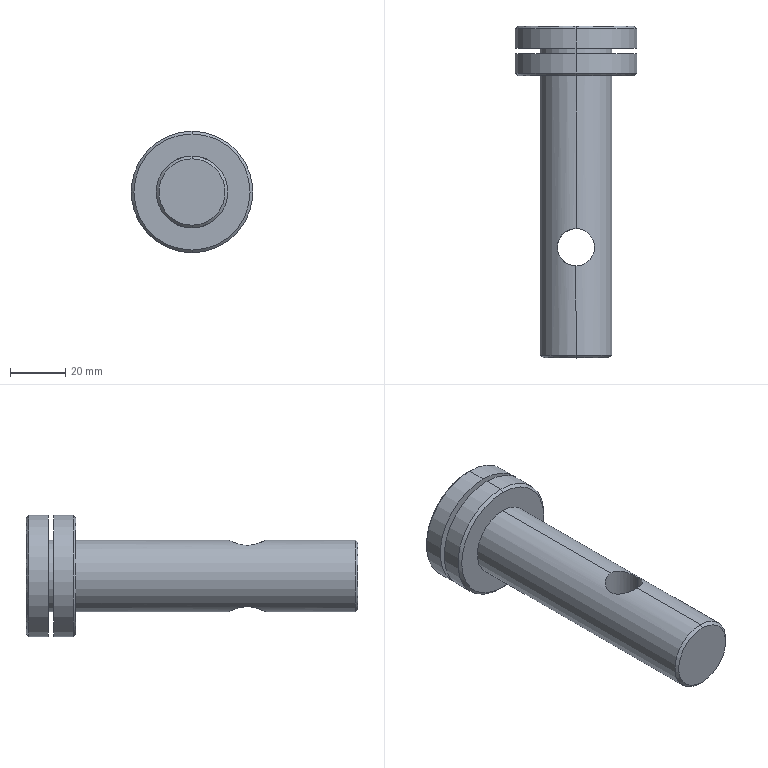Part | SolidWorks | features 3DProfileFeature 1, Chamfer 1, CirPattern 1, HoleWzd 1, ICE 1, Revolution 1 | 1 solid | 37 faces | box 44 x 120 x 44 mm | volume 75501 mm3 | cylinder 18 | cone 14 | plane 5 | commonest cylinder face diameters 3.3 x8 26 x4 44 x4 13.5 x2
STEP:
#1=CARTESIAN_POINT('',(-6.75,40.,-11.11));
#2=VERTEX_POINT('',#1);
#3=CARTESIAN_POINT('',(0.,33.25,-13.));
#4=VERTEX_POINT('',#3);
#5=CARTESIAN_POINT('',(-6.75,40.,-11.11));
#6=CARTESIAN_POINT('',(-6.75,39.775,-11.11));
#7=CARTESIAN_POINT('',(-6.739,39.547,-11.117));
#8=CARTESIAN_POINT('',(-6.693,39.098,-11.145));
#9=CARTESIAN_POINT('',(-6.66,38.877,-11.165));
#10=CARTESIAN_POINT('',(-6.571,38.44,-11.217));
#11=CARTESIAN_POINT('',(-6.516,38.224,-11.249));
#12=CARTESIAN_POINT('',(-6.385,37.799,-11.324));
#13=CARTESIAN_POINT('',(-6.308,37.589,-11.367));
#14=CARTESIAN_POINT('',(-6.051,36.977,-11.507));
#15=CARTESIAN_POINT('',(-5.844,36.593,-11.616));
#16=CARTESIAN_POINT('',(-5.478,36.051,-11.79));
#17=CARTESIAN_POINT('',(-5.347,35.874,-11.85));
#18=CARTESIAN_POINT('',(-5.07,35.539,-11.971));
#19=CARTESIAN_POINT('',(-4.925,35.379,-12.032));
#20=CARTESIAN_POINT('',(-4.466,34.92,-12.213));
#21=CARTESIAN_POINT('',(-4.132,34.644,-12.332));
#22=CARTESIAN_POINT('',(-3.4,34.152,-12.553));
#23=CARTESIAN_POINT('',(-3.015,33.945,-12.652));
#24=CARTESIAN_POINT('',(-2.408,33.69,-12.777));
#25=CARTESIAN_POINT('',(-2.2,33.615,-12.814));
#26=CARTESIAN_POINT('',(-1.775,33.484,-12.88));
#27=CARTESIAN_POINT('',(-1.555,33.428,-12.909));
#28=CARTESIAN_POINT('',(-0.8938,33.294,-12.977));
#29=CARTESIAN_POINT('',(-0.4489,33.25,-13.));
#30=CARTESIAN_POINT('',(0.,33.25,-13.));
#31=B_SPLINE_CURVE_WITH_KNOTS('',3,(#5,#6,#7,#8,#9,#10,#11,#12,#13,#14,#15,#16,#17,#18,#19,#20,#21,#22,#23,#24,#25,#26,#27,#28,#29,#30),.UNSPECIFIED.,.F.,.F.,(4,2,2,2,2,2,2,2,2,2,2,2,4),(0.01076,0.01143,0.0121,0.01277,0.01345,0.01479,0.01546,0.01613,0.01747,0.01882,0.01949,0.02016,0.0215),.UNSPECIFIED.);
#32=EDGE_CURVE('',#2,#4,#31,.T.);
#33=ORIENTED_EDGE('',*,*,#32,.F.);
#34=CARTESIAN_POINT('',(-6.75,40.,11.11));
#35=VERTEX_POINT('',#34);
#36=CARTESIAN_POINT('',(-6.75,40.,-22.));
#37=DIRECTION('',(0.,0.,1.));
#38=VECTOR('',#37,1000.);
#39=LINE('',#36,#38);
#40=EDGE_CURVE('',#2,#35,#39,.T.);
#41=ORIENTED_EDGE('',*,*,#40,.T.);
#42=CARTESIAN_POINT('',(0.,33.25,13.));
#43=VERTEX_POINT('',#42);
#44=CARTESIAN_POINT('',(0.,33.25,13.));
#45=CARTESIAN_POINT('',(-0.2253,33.25,13.));
#46=CARTESIAN_POINT('',(-0.4536,33.261,12.994));
#47=CARTESIAN_POINT('',(-0.9024,33.307,12.971));
#48=CARTESIAN_POINT('',(-1.124,33.34,12.953));
#49=CARTESIAN_POINT('',(-1.561,33.429,12.908));
#50=CARTESIAN_POINT('',(-1.777,33.484,12.88));
#51=CARTESIAN_POINT('',(-2.204,33.616,12.814));
#52=CARTESIAN_POINT('',(-2.415,33.693,12.775));
#53=CARTESIAN_POINT('',(-3.029,33.951,12.649));
#54=CARTESIAN_POINT('',(-3.414,34.161,12.549));
#55=CARTESIAN_POINT('',(-3.958,34.528,12.384));
#56=CARTESIAN_POINT('',(-4.134,34.66,12.326));
#57=CARTESIAN_POINT('',(-4.471,34.938,12.208));
#58=CARTESIAN_POINT('',(-4.631,35.084,12.148));
#59=CARTESIAN_POINT('',(-5.088,35.544,11.967));
#60=CARTESIAN_POINT('',(-5.363,35.878,11.845));
#61=CARTESIAN_POINT('',(-5.852,36.607,11.612));
#62=CARTESIAN_POINT('',(-6.058,36.991,11.504));
#63=CARTESIAN_POINT('',(-6.311,37.597,11.366));
#64=CARTESIAN_POINT('',(-6.386,37.803,11.323));
#65=CARTESIAN_POINT('',(-6.517,38.228,11.249));
#66=CARTESIAN_POINT('',(-6.573,38.447,11.216));
#67=CARTESIAN_POINT('',(-6.706,39.107,11.137));
#68=CARTESIAN_POINT('',(-6.75,39.552,11.11));
#69=CARTESIAN_POINT('',(-6.75,40.,11.11));
#70=B_SPLINE_CURVE_WITH_KNOTS('',3,(#44,#45,#46,#47,#48,#49,#50,#51,#52,#53,#54,#55,#56,#57,#58,#59,#60,#61,#62,#63,#64,#65,#66,#67,#68,#69),.UNSPECIFIED.,.F.,.F.,(4,2,2,2,2,2,2,2,2,2,2,2,4),(0.01076,0.01143,0.0121,0.01277,0.01344,0.01479,0.01546,0.01613,0.01747,0.01881,0.01949,0.02016,0.0215),.UNSPECIFIED.);
#71=EDGE_CURVE('',#43,#35,#70,.T.);
#72=ORIENTED_EDGE('',*,*,#71,.F.);
#73=CARTESIAN_POINT('',(6.75,40.,11.11));
#74=VERTEX_POINT('',#73);
#75=CARTESIAN_POINT('',(6.75,40.,11.11));
#76=CARTESIAN_POINT('',(6.75,39.545,11.11));
#77=CARTESIAN_POINT('',(6.704,39.099,11.138));
#78=CARTESIAN_POINT('',(6.528,38.225,11.243));
#79=CARTESIAN_POINT('',(6.394,37.793,11.32));
#80=CARTESIAN_POINT('',(6.053,36.981,11.506));
#81=CARTESIAN_POINT('',(5.846,36.597,11.615));
#82=CARTESIAN_POINT('',(5.357,35.87,11.848));
#83=CARTESIAN_POINT('',(5.08,35.534,11.971));
#84=CARTESIAN_POINT('',(4.621,35.075,12.152));
#85=CARTESIAN_POINT('',(4.461,34.929,12.212));
#86=CARTESIAN_POINT('',(4.125,34.652,12.33));
#87=CARTESIAN_POINT('',(3.948,34.52,12.388));
#88=CARTESIAN_POINT('',(3.402,34.154,12.553));
#89=CARTESIAN_POINT('',(3.018,33.946,12.652));
#90=CARTESIAN_POINT('',(2.409,33.691,12.776));
#91=CARTESIAN_POINT('',(2.201,33.615,12.814));
#92=CARTESIAN_POINT('',(1.772,33.483,12.88));
#93=CARTESIAN_POINT('',(1.553,33.427,12.909));
#94=CARTESIAN_POINT('',(0.8956,33.295,12.977));
#95=CARTESIAN_POINT('',(0.451,33.25,13.));
#96=CARTESIAN_POINT('',(0.,33.25,13.));
#97=B_SPLINE_CURVE_WITH_KNOTS('',3,(#75,#76,#77,#78,#79,#80,#81,#82,#83,#84,#85,#86,#87,#88,#89,#90,#91,#92,#93,#94,#95,#96),.UNSPECIFIED.,.F.,.F.,(4,2,2,2,2,2,2,2,2,2,4),(0.,0.001344,0.002689,0.004033,0.005378,0.00605,0.006722,0.008066,0.008739,0.009411,0.01076),.UNSPECIFIED.);
#98=EDGE_CURVE('',#74,#43,#97,.T.);
#99=ORIENTED_EDGE('',*,*,#98,.F.);
#100=CARTESIAN_POINT('',(6.75,40.,-11.11));
#101=VERTEX_POINT('',#100);
#102=CARTESIAN_POINT('',(6.75,40.,-22.));
#103=DIRECTION('',(0.,0.,1.));
#104=VECTOR('',#103,1000.);
#105=LINE('',#102,#104);
#106=EDGE_CURVE('',#101,#74,#105,.T.);
#107=ORIENTED_EDGE('',*,*,#106,.F.);
#108=CARTESIAN_POINT('',(0.,33.25,-13.));
#109=CARTESIAN_POINT('',(0.4487,33.25,-13.));
#110=CARTESIAN_POINT('',(0.9051,33.296,-12.976));
#111=CARTESIAN_POINT('',(1.781,33.474,-12.885));
#112=CARTESIAN_POINT('',(2.207,33.605,-12.818));
#113=CARTESIAN_POINT('',(3.029,33.951,-12.649));
#114=CARTESIAN_POINT('',(3.414,34.161,-12.549));
#115=CARTESIAN_POINT('',(4.138,34.649,-12.33));
#116=CARTESIAN_POINT('',(4.478,34.93,-12.209));
#117=CARTESIAN_POINT('',(5.089,35.544,-11.967));
#118=CARTESIAN_POINT('',(5.363,35.878,-11.845));
#119=CARTESIAN_POINT('',(5.728,36.422,-11.671));
#120=CARTESIAN_POINT('',(5.842,36.611,-11.614));
#121=CARTESIAN_POINT('',(6.049,36.996,-11.508));
#122=CARTESIAN_POINT('',(6.143,37.194,-11.458));
#123=CARTESIAN_POINT('',(6.396,37.799,-11.319));
#124=CARTESIAN_POINT('',(6.527,38.22,-11.243));
#125=CARTESIAN_POINT('',(6.706,39.105,-11.138));
#126=CARTESIAN_POINT('',(6.75,39.553,-11.11));
#127=CARTESIAN_POINT('',(6.75,40.,-11.11));
#128=B_SPLINE_CURVE_WITH_KNOTS('',3,(#108,#109,#110,#111,#112,#113,#114,#115,#116,#117,#118,#119,#120,#121,#122,#123,#124,#125,#126,#127),.UNSPECIFIED.,.F.,.F.,(4,2,2,2,2,2,2,2,2,4),(0.0215,0.02285,0.02419,0.02553,0.02687,0.02822,0.02889,0.02956,0.0309,0.03224),.UNSPECIFIED.);
#129=EDGE_CURVE('',#4,#101,#128,.T.);
#130=ORIENTED_EDGE('',*,*,#129,.F.);
#131=EDGE_LOOP('',(#33,#41,#72,#99,#107,#130));
#132=FACE_OUTER_BOUND('',#131,.T.);
#133=CARTESIAN_POINT('',(0.,40.,-22.));
#134=DIRECTION('',(0.,0.,1.));
#135=DIRECTION('',(1.,0.,0.));
#136=AXIS2_PLACEMENT_3D('',#133,#134,#135);
#137=CYLINDRICAL_SURFACE('',#136,6.75);
#138=ADVANCED_FACE('',(#132),#137,.F.);
#139=CARTESIAN_POINT('',(15.,119.625,-1.65));
#140=VERTEX_POINT('',#139);
#141=CARTESIAN_POINT('',(15.,119.625,1.65));
#142=VERTEX_POINT('',#141);
#143=CARTESIAN_POINT('',(15.,119.625,0.));
#144=DIRECTION('',(0.,1.,0.));
#145=DIRECTION('',(0.,0.,1.));
#146=AXIS2_PLACEMENT_3D('',#143,#144,#145);
#147=CIRCLE('',#146,1.65);
#148=EDGE_CURVE('',#140,#142,#147,.T.);
#149=ORIENTED_EDGE('',*,*,#148,.F.);
#150=CARTESIAN_POINT('',(15.,120.,-2.025));
#151=VERTEX_POINT('',#150);
#152=CARTESIAN_POINT('',(15.,120.,-2.025));
#153=DIRECTION('',(0.,0.7071,-0.7071));
#154=VECTOR('',#153,1000.);
#155=LINE('',#152,#154);
#156=EDGE_CURVE('',#140,#151,#155,.T.);
#157=ORIENTED_EDGE('',*,*,#156,.T.);
#158=CARTESIAN_POINT('',(15.,120.,2.025));
#159=VERTEX_POINT('',#158);
#160=CARTESIAN_POINT('',(15.,120.,0.));
#161=DIRECTION('',(0.,1.,0.));
#162=DIRECTION('',(0.,0.,1.));
#163=AXIS2_PLACEMENT_3D('',#160,#161,#162);
#164=CIRCLE('',#163,2.025);
#165=EDGE_CURVE('',#151,#159,#164,.T.);
#166=ORIENTED_EDGE('',*,*,#165,.T.);
#167=CARTESIAN_POINT('',(15.,120.,2.025));
#168=DIRECTION('',(0.,0.7071,0.7071));
#169=VECTOR('',#168,1000.);
#170=LINE('',#167,#169);
#171=EDGE_CURVE('',#142,#159,#170,.T.);
#172=ORIENTED_EDGE('',*,*,#171,.F.);
#173=EDGE_LOOP('',(#149,#157,#166,#172));
#174=FACE_OUTER_BOUND('',#173,.T.);
#175=CARTESIAN_POINT('',(15.,120.,0.));
#176=DIRECTION('',(0.,1.,0.));
#177=DIRECTION('',(0.,0.,1.));
#178=AXIS2_PLACEMENT_3D('',#175,#176,#177);
#179=CONICAL_SURFACE('',#178,2.025,0.7854);
#180=ADVANCED_FACE('',(#174),#179,.F.);
#181=CARTESIAN_POINT('',(15.,112.,-1.65));
#182=VERTEX_POINT('',#181);
#183=CARTESIAN_POINT('',(15.,112.,1.65));
#184=VERTEX_POINT('',#183);
#185=CARTESIAN_POINT('',(15.,112.,0.));
#186=DIRECTION('',(0.,1.,0.));
#187=DIRECTION('',(0.,0.,1.));
#188=AXIS2_PLACEMENT_3D('',#185,#186,#187);
#189=CIRCLE('',#188,1.65);
#190=EDGE_CURVE('',#182,#184,#189,.T.);
#191=ORIENTED_EDGE('',*,*,#190,.F.);
#192=CARTESIAN_POINT('',(15.,120.,-1.65));
#193=DIRECTION('',(0.,1.,0.));
#194=VECTOR('',#193,1000.);
#195=LINE('',#192,#194);
#196=EDGE_CURVE('',#182,#140,#195,.T.);
#197=ORIENTED_EDGE('',*,*,#196,.T.);
#198=ORIENTED_EDGE('',*,*,#148,.T.);
#199=CARTESIAN_POINT('',(15.,120.,1.65));
#200=DIRECTION('',(0.,1.,0.));
#201=VECTOR('',#200,1000.);
#202=LINE('',#199,#201);
#203=EDGE_CURVE('',#184,#142,#202,.T.);
#204=ORIENTED_EDGE('',*,*,#203,.F.);
#205=EDGE_LOOP('',(#191,#197,#198,#204));
#206=FACE_OUTER_BOUND('',#205,.T.);
#207=CARTESIAN_POINT('',(15.,120.,0.));
#208=DIRECTION('',(0.,1.,0.));
#209=DIRECTION('',(0.,0.,1.));
#210=AXIS2_PLACEMENT_3D('',#207,#208,#209);
#211=CYLINDRICAL_SURFACE('',#210,1.65);
#212=ADVANCED_FACE('',(#206),#211,.F.);
#213=CARTESIAN_POINT('',(0.,119.625,13.35));
#214=VERTEX_POINT('',#213);
#215=CARTESIAN_POINT('',(0.,119.625,16.65));
#216=VERTEX_POINT('',#215);
#217=CARTESIAN_POINT('',(0.,119.625,15.));
#218=DIRECTION('',(0.,1.,0.));
#219=DIRECTION('',(0.,0.,1.));
#220=AXIS2_PLACEMENT_3D('',#217,#218,#219);
#221=CIRCLE('',#220,1.65);
#222=EDGE_CURVE('',#214,#216,#221,.T.);
#223=ORIENTED_EDGE('',*,*,#222,.F.);
#224=CARTESIAN_POINT('',(0.,120.,12.975));
#225=VERTEX_POINT('',#224);
#226=CARTESIAN_POINT('',(0.,120.,12.975));
#227=DIRECTION('',(0.,0.7071,-0.7071));
#228=VECTOR('',#227,1000.);
#229=LINE('',#226,#228);
#230=EDGE_CURVE('',#214,#225,#229,.T.);
#231=ORIENTED_EDGE('',*,*,#230,.T.);
#232=CARTESIAN_POINT('',(0.,120.,17.025));
#233=VERTEX_POINT('',#232);
#234=CARTESIAN_POINT('',(0.,120.,15.));
#235=DIRECTION('',(0.,1.,0.));
#236=DIRECTION('',(0.,0.,1.));
#237=AXIS2_PLACEMENT_3D('',#234,#235,#236);
#238=CIRCLE('',#237,2.025);
#239=EDGE_CURVE('',#225,#233,#238,.T.);
#240=ORIENTED_EDGE('',*,*,#239,.T.);
#241=CARTESIAN_POINT('',(0.,120.,17.025));
#242=DIRECTION('',(0.,0.7071,0.7071));
#243=VECTOR('',#242,1000.);
#244=LINE('',#241,#243);
#245=EDGE_CURVE('',#216,#233,#244,.T.);
#246=ORIENTED_EDGE('',*,*,#245,.F.);
#247=EDGE_LOOP('',(#223,#231,#240,#246));
#248=FACE_OUTER_BOUND('',#247,.T.);
#249=CARTESIAN_POINT('',(0.,120.,15.));
#250=DIRECTION('',(0.,1.,0.));
#251=DIRECTION('',(0.,0.,1.));
#252=AXIS2_PLACEMENT_3D('',#249,#250,#251);
#253=CONICAL_SURFACE('',#252,2.025,0.7854);
#254=ADVANCED_FACE('',(#248),#253,.F.);
#255=CARTESIAN_POINT('',(0.,112.,13.35));
#256=VERTEX_POINT('',#255);
#257=CARTESIAN_POINT('',(0.,112.,16.65));
#258=VERTEX_POINT('',#257);
#259=CARTESIAN_POINT('',(0.,112.,15.));
#260=DIRECTION('',(0.,1.,0.));
#261=DIRECTION('',(0.,0.,1.));
#262=AXIS2_PLACEMENT_3D('',#259,#260,#261);
#263=CIRCLE('',#262,1.65);
#264=EDGE_CURVE('',#256,#258,#263,.T.);
#265=ORIENTED_EDGE('',*,*,#264,.F.);
#266=CARTESIAN_POINT('',(0.,120.,13.35));
#267=DIRECTION('',(0.,1.,0.));
#268=VECTOR('',#267,1000.);
#269=LINE('',#266,#268);
#270=EDGE_CURVE('',#256,#214,#269,.T.);
#271=ORIENTED_EDGE('',*,*,#270,.T.);
#272=ORIENTED_EDGE('',*,*,#222,.T.);
#273=CARTESIAN_POINT('',(0.,120.,16.65));
#274=DIRECTION('',(0.,1.,0.));
#275=VECTOR('',#274,1000.);
#276=LINE('',#273,#275);
#277=EDGE_CURVE('',#258,#216,#276,.T.);
#278=ORIENTED_EDGE('',*,*,#277,.F.);
#279=EDGE_LOOP('',(#265,#271,#272,#278));
#280=FACE_OUTER_BOUND('',#279,.T.);
#281=CARTESIAN_POINT('',(0.,120.,15.));
#282=DIRECTION('',(0.,1.,0.));
#283=DIRECTION('',(0.,0.,1.));
#284=AXIS2_PLACEMENT_3D('',#281,#282,#283);
#285=CYLINDRICAL_SURFACE('',#284,1.65);
#286=ADVANCED_FACE('',(#280),#285,.F.);
#287=CARTESIAN_POINT('',(-15.,119.625,-1.65));
#288=VERTEX_POINT('',#287);
#289=CARTESIAN_POINT('',(-15.,119.625,1.65));
#290=VERTEX_POINT('',#289);
#291=CARTESIAN_POINT('',(-15.,119.625,0.));
#292=DIRECTION('',(0.,1.,0.));
#293=DIRECTION('',(0.,0.,1.));
#294=AXIS2_PLACEMENT_3D('',#291,#292,#293);
#295=CIRCLE('',#294,1.65);
#296=EDGE_CURVE('',#288,#290,#295,.T.);
#297=ORIENTED_EDGE('',*,*,#296,.F.);
#298=CARTESIAN_POINT('',(-15.,120.,-2.025));
#299=VERTEX_POINT('',#298);
#300=CARTESIAN_POINT('',(-15.,120.,-2.025));
#301=DIRECTION('',(0.,0.7071,-0.7071));
#302=VECTOR('',#301,1000.);
#303=LINE('',#300,#302);
#304=EDGE_CURVE('',#288,#299,#303,.T.);
#305=ORIENTED_EDGE('',*,*,#304,.T.);
#306=CARTESIAN_POINT('',(-15.,120.,2.025));
#307=VERTEX_POINT('',#306);
#308=CARTESIAN_POINT('',(-15.,120.,0.));
#309=DIRECTION('',(0.,1.,0.));
#310=DIRECTION('',(0.,0.,1.));
#311=AXIS2_PLACEMENT_3D('',#308,#309,#310);
#312=CIRCLE('',#311,2.025);
#313=EDGE_CURVE('',#299,#307,#312,.T.);
#314=ORIENTED_EDGE('',*,*,#313,.T.);
#315=CARTESIAN_POINT('',(-15.,120.,2.025));
#316=DIRECTION('',(0.,0.7071,0.7071));
#317=VECTOR('',#316,1000.);
#318=LINE('',#315,#317);
#319=EDGE_CURVE('',#290,#307,#318,.T.);
#320=ORIENTED_EDGE('',*,*,#319,.F.);
#321=EDGE_LOOP('',(#297,#305,#314,#320));
#322=FACE_OUTER_BOUND('',#321,.T.);
#323=CARTESIAN_POINT('',(-15.,120.,0.));
#324=DIRECTION('',(0.,1.,0.));
#325=DIRECTION('',(0.,0.,1.));
#326=AXIS2_PLACEMENT_3D('',#323,#324,#325);
#327=CONICAL_SURFACE('',#326,2.025,0.7854);
#328=ADVANCED_FACE('',(#322),#327,.F.);
#329=CARTESIAN_POINT('',(-15.,112.,-1.65));
#330=VERTEX_POINT('',#329);
#331=CARTESIAN_POINT('',(-15.,112.,1.65));
#332=VERTEX_POINT('',#331);
#333=CARTESIAN_POINT('',(-15.,112.,0.));
#334=DIRECTION('',(0.,1.,0.));
#335=DIRECTION('',(0.,0.,1.));
#336=AXIS2_PLACEMENT_3D('',#333,#334,#335);
#337=CIRCLE('',#336,1.65);
#338=EDGE_CURVE('',#330,#332,#337,.T.);
#339=ORIENTED_EDGE('',*,*,#338,.F.);
#340=CARTESIAN_POINT('',(-15.,120.,-1.65));
#341=DIRECTION('',(0.,1.,0.));
#342=VECTOR('',#341,1000.);
#343=LINE('',#340,#342);
#344=EDGE_CURVE('',#330,#288,#343,.T.);
#345=ORIENTED_EDGE('',*,*,#344,.T.);
#346=ORIENTED_EDGE('',*,*,#296,.T.);
#347=CARTESIAN_POINT('',(-15.,120.,1.65));
#348=DIRECTION('',(0.,1.,0.));
#349=VECTOR('',#348,1000.);
#350=LINE('',#347,#349);
#351=EDGE_CURVE('',#332,#290,#350,.T.);
#352=ORIENTED_EDGE('',*,*,#351,.F.);
#353=EDGE_LOOP('',(#339,#345,#346,#352));
#354=FACE_OUTER_BOUND('',#353,.T.);
#355=CARTESIAN_POINT('',(-15.,120.,0.));
#356=DIRECTION('',(0.,1.,0.));
#357=DIRECTION('',(0.,0.,1.));
#358=AXIS2_PLACEMENT_3D('',#355,#356,#357);
#359=CYLINDRICAL_SURFACE('',#358,1.65);
#360=ADVANCED_FACE('',(#354),#359,.F.);
#361=CARTESIAN_POINT('',(0.,119.625,-16.65));
#362=VERTEX_POINT('',#361);
#363=CARTESIAN_POINT('',(0.,119.625,-13.35));
#364=VERTEX_POINT('',#363);
#365=CARTESIAN_POINT('',(0.,119.625,-15.));
#366=DIRECTION('',(0.,1.,0.));
#367=DIRECTION('',(0.,0.,1.));
#368=AXIS2_PLACEMENT_3D('',#365,#366,#367);
#369=CIRCLE('',#368,1.65);
#370=EDGE_CURVE('',#362,#364,#369,.T.);
#371=ORIENTED_EDGE('',*,*,#370,.F.);
#372=CARTESIAN_POINT('',(0.,120.,-17.025));
#373=VERTEX_POINT('',#372);
#374=CARTESIAN_POINT('',(0.,120.,-17.025));
#375=DIRECTION('',(0.,0.7071,-0.7071));
#376=VECTOR('',#375,1000.);
#377=LINE('',#374,#376);
#378=EDGE_CURVE('',#362,#373,#377,.T.);
#379=ORIENTED_EDGE('',*,*,#378,.T.);
#380=CARTESIAN_POINT('',(0.,120.,-12.975));
#381=VERTEX_POINT('',#380);
#382=CARTESIAN_POINT('',(0.,120.,-15.));
#383=DIRECTION('',(0.,1.,0.));
#384=DIRECTION('',(0.,0.,1.));
#385=AXIS2_PLACEMENT_3D('',#382,#383,#384);
#386=CIRCLE('',#385,2.025);
#387=EDGE_CURVE('',#373,#381,#386,.T.);
#388=ORIENTED_EDGE('',*,*,#387,.T.);
#389=CARTESIAN_POINT('',(0.,120.,-12.975));
#390=DIRECTION('',(0.,0.7071,0.7071));
#391=VECTOR('',#390,1000.);
#392=LINE('',#389,#391);
#393=EDGE_CURVE('',#364,#381,#392,.T.);
#394=ORIENTED_EDGE('',*,*,#393,.F.);
#395=EDGE_LOOP('',(#371,#379,#388,#394));
#396=FACE_OUTER_BOUND('',#395,.T.);
#397=CARTESIAN_POINT('',(0.,120.,-15.));
#398=DIRECTION('',(0.,1.,0.));
#399=DIRECTION('',(0.,0.,1.));
#400=AXIS2_PLACEMENT_3D('',#397,#398,#399);
#401=CONICAL_SURFACE('',#400,2.025,0.7854);
#402=ADVANCED_FACE('',(#396),#401,.F.);
#403=CARTESIAN_POINT('',(0.,112.,-16.65));
#404=VERTEX_POINT('',#403);
#405=CARTESIAN_POINT('',(0.,112.,-13.35));
#406=VERTEX_POINT('',#405);
#407=CARTESIAN_POINT('',(0.,112.,-15.));
#408=DIRECTION('',(0.,1.,0.));
#409=DIRECTION('',(0.,0.,1.));
#410=AXIS2_PLACEMENT_3D('',#407,#408,#409);
#411=CIRCLE('',#410,1.65);
#412=EDGE_CURVE('',#404,#406,#411,.T.);
#413=ORIENTED_EDGE('',*,*,#412,.F.);
#414=CARTESIAN_POINT('',(0.,120.,-16.65));
#415=DIRECTION('',(0.,1.,0.));
#416=VECTOR('',#415,1000.);
#417=LINE('',#414,#416);
#418=EDGE_CURVE('',#404,#362,#417,.T.);
#419=ORIENTED_EDGE('',*,*,#418,.T.);
#420=ORIENTED_EDGE('',*,*,#370,.T.);
#421=CARTESIAN_POINT('',(0.,120.,-13.35));
#422=DIRECTION('',(0.,1.,0.));
#423=VECTOR('',#422,1000.);
#424=LINE('',#421,#423);
#425=EDGE_CURVE('',#406,#364,#424,.T.);
#426=ORIENTED_EDGE('',*,*,#425,.F.);
#427=EDGE_LOOP('',(#413,#419,#420,#426));
#428=FACE_OUTER_BOUND('',#427,.T.);
#429=CARTESIAN_POINT('',(0.,120.,-15.));
#430=DIRECTION('',(0.,1.,0.));
#431=DIRECTION('',(0.,0.,1.));
#432=AXIS2_PLACEMENT_3D('',#429,#430,#431);
#433=CYLINDRICAL_SURFACE('',#432,1.65);
#434=ADVANCED_FACE('',(#428),#433,.F.);
#435=CARTESIAN_POINT('',(0.,102.,-21.));
#436=VERTEX_POINT('',#435);
#437=CARTESIAN_POINT('',(0.,102.,21.));
#438=VERTEX_POINT('',#437);
#439=CARTESIAN_POINT('',(0.,102.,0.));
#440=DIRECTION('',(0.,-1.,0.));
#441=DIRECTION('',(0.,0.,1.));
#442=AXIS2_PLACEMENT_3D('',#439,#440,#441);
#443=CIRCLE('',#442,21.);
#444=EDGE_CURVE('',#436,#438,#443,.T.);
#445=ORIENTED_EDGE('',*,*,#444,.F.);
#446=CARTESIAN_POINT('',(0.,103.,-22.));
#447=VERTEX_POINT('',#446);
#448=CARTESIAN_POINT('',(0.,102.,-21.));
#449=DIRECTION('',(0.,0.7071,-0.7071));
#450=VECTOR('',#449,1000.);
#451=LINE('',#448,#450);
#452=EDGE_CURVE('',#436,#447,#451,.T.);
#453=ORIENTED_EDGE('',*,*,#452,.T.);
#454=CARTESIAN_POINT('',(0.,103.,22.));
#455=VERTEX_POINT('',#454);
#456=CARTESIAN_POINT('',(0.,103.,0.));
#457=DIRECTION('',(0.,1.,0.));
#458=DIRECTION('',(0.,0.,1.));
#459=AXIS2_PLACEMENT_3D('',#456,#457,#458);
#460=CIRCLE('',#459,22.);
#461=EDGE_CURVE('',#455,#447,#460,.T.);
#462=ORIENTED_EDGE('',*,*,#461,.F.);
#463=CARTESIAN_POINT('',(0.,102.,21.));
#464=DIRECTION('',(0.,0.7071,0.7071));
#465=VECTOR('',#464,1000.);
#466=LINE('',#463,#465);
#467=EDGE_CURVE('',#438,#455,#466,.T.);
#468=ORIENTED_EDGE('',*,*,#467,.F.);
#469=EDGE_LOOP('',(#445,#453,#462,#468));
#470=FACE_OUTER_BOUND('',#469,.T.);
#471=CARTESIAN_POINT('',(0.,102.,0.));
#472=DIRECTION('',(0.,1.,0.));
#473=DIRECTION('',(0.,0.,1.));
#474=AXIS2_PLACEMENT_3D('',#471,#472,#473);
#475=CONICAL_SURFACE('',#474,21.,0.7854);
#476=ADVANCED_FACE('',(#470),#475,.T.);
#477=CARTESIAN_POINT('',(0.,0.,-12.));
#478=VERTEX_POINT('',#477);
#479=CARTESIAN_POINT('',(0.,0.,12.));
#480=VERTEX_POINT('',#479);
#481=CARTESIAN_POINT('',(0.,0.,0.));
#482=DIRECTION('',(0.,-1.,0.));
#483=DIRECTION('',(0.,0.,1.));
#484=AXIS2_PLACEMENT_3D('',#481,#482,#483);
#485=CIRCLE('',#484,12.);
#486=EDGE_CURVE('',#478,#480,#485,.T.);
#487=ORIENTED_EDGE('',*,*,#486,.F.);
#488=CARTESIAN_POINT('',(0.,1.,-13.));
#489=VERTEX_POINT('',#488);
#490=CARTESIAN_POINT('',(0.,0.,-12.));
#491=DIRECTION('',(0.,0.7071,-0.7071));
#492=VECTOR('',#491,1000.);
#493=LINE('',#490,#492);
#494=EDGE_CURVE('',#478,#489,#493,.T.);
#495=ORIENTED_EDGE('',*,*,#494,.T.);
#496=CARTESIAN_POINT('',(0.,1.,13.));
#497=VERTEX_POINT('',#496);
#498=CARTESIAN_POINT('',(0.,1.,0.));
#499=DIRECTION('',(0.,1.,0.));
#500=DIRECTION('',(0.,0.,1.));
#501=AXIS2_PLACEMENT_3D('',#498,#499,#500);
#502=CIRCLE('',#501,13.);
#503=EDGE_CURVE('',#497,#489,#502,.T.);
#504=ORIENTED_EDGE('',*,*,#503,.F.);
#505=CARTESIAN_POINT('',(0.,0.,12.));
#506=DIRECTION('',(0.,0.7071,0.7071));
#507=VECTOR('',#506,1000.);
#508=LINE('',#505,#507);
#509=EDGE_CURVE('',#480,#497,#508,.T.);
#510=ORIENTED_EDGE('',*,*,#509,.F.);
#511=EDGE_LOOP('',(#487,#495,#504,#510));
#512=FACE_OUTER_BOUND('',#511,.T.);
#513=CARTESIAN_POINT('',(0.,0.,0.));
#514=DIRECTION('',(0.,1.,0.));
#515=DIRECTION('',(0.,0.,1.));
#516=AXIS2_PLACEMENT_3D('',#513,#514,#515);
#517=CONICAL_SURFACE('',#516,12.,0.7854);
#518=ADVANCED_FACE('',(#512),#517,.T.);
#519=CARTESIAN_POINT('',(0.,120.,21.));
#520=VERTEX_POINT('',#519);
#521=CARTESIAN_POINT('',(0.,120.,-21.));
#522=VERTEX_POINT('',#521);
#523=CARTESIAN_POINT('',(0.,120.,0.));
#524=DIRECTION('',(0.,1.,0.));
#525=DIRECTION('',(0.,0.,-1.));
#526=AXIS2_PLACEMENT_3D('',#523,#524,#525);
#527=CIRCLE('',#526,21.);
#528=EDGE_CURVE('',#520,#522,#527,.T.);
#529=ORIENTED_EDGE('',*,*,#528,.F.);
#530=CARTESIAN_POINT('',(0.,119.,22.));
#531=VERTEX_POINT('',#530);
#532=CARTESIAN_POINT('',(0.,119.,22.));
#533=DIRECTION('',(0.,-0.7071,0.7071));
#534=VECTOR('',#533,1000.);
#535=LINE('',#532,#534);
#536=EDGE_CURVE('',#520,#531,#535,.T.);
#537=ORIENTED_EDGE('',*,*,#536,.T.);
#538=CARTESIAN_POINT('',(0.,119.,-22.));
#539=VERTEX_POINT('',#538);
#540=CARTESIAN_POINT('',(0.,119.,0.));
#541=DIRECTION('',(0.,-1.,0.));
#542=DIRECTION('',(0.,0.,-1.));
#543=AXIS2_PLACEMENT_3D('',#540,#541,#542);
#544=CIRCLE('',#543,22.);
#545=EDGE_CURVE('',#539,#531,#544,.T.);
#546=ORIENTED_EDGE('',*,*,#545,.F.);
#547=CARTESIAN_POINT('',(0.,119.,-22.));
#548=DIRECTION('',(0.,-0.7071,-0.7071));
#549=VECTOR('',#548,1000.);
#550=LINE('',#547,#549);
#551=EDGE_CURVE('',#522,#539,#550,.T.);
#552=ORIENTED_EDGE('',*,*,#551,.F.);
#553=EDGE_LOOP('',(#529,#537,#546,#552));
#554=FACE_OUTER_BOUND('',#553,.T.);
#555=CARTESIAN_POINT('',(0.,119.,0.));
#556=DIRECTION('',(0.,-1.,0.));
#557=DIRECTION('',(0.,0.,-1.));
#558=AXIS2_PLACEMENT_3D('',#555,#556,#557);
#559=CONICAL_SURFACE('',#558,22.,0.7854);
#560=ADVANCED_FACE('',(#554),#559,.T.);
#561=CARTESIAN_POINT('',(0.,102.,-13.));
#562=VERTEX_POINT('',#561);
#563=CARTESIAN_POINT('',(0.,102.,13.));
#564=VERTEX_POINT('',#563);
#565=CARTESIAN_POINT('',(0.,102.,0.));
#566=DIRECTION('',(0.,-1.,0.));
#567=DIRECTION('',(0.,0.,-1.));
#568=AXIS2_PLACEMENT_3D('',#565,#566,#567);
#569=CIRCLE('',#568,13.);
#570=EDGE_CURVE('',#562,#564,#569,.T.);
#571=ORIENTED_EDGE('',*,*,#570,.T.);
#572=CARTESIAN_POINT('',(0.,46.75,13.));
#573=VERTEX_POINT('',#572);
#574=CARTESIAN_POINT('',(0.,0.,13.));
#575=DIRECTION('',(0.,-1.,0.));
#576=VECTOR('',#575,1000.);
#577=LINE('',#574,#576);
#578=EDGE_CURVE('',#564,#573,#577,.T.);
#579=ORIENTED_EDGE('',*,*,#578,.T.);
#580=CARTESIAN_POINT('',(0.,46.75,13.));
#581=CARTESIAN_POINT('',(0.2237,46.75,13.));
#582=CARTESIAN_POINT('',(0.4478,46.739,12.994));
#583=CARTESIAN_POINT('',(0.8971,46.694,12.971));
#584=CARTESIAN_POINT('',(1.122,46.66,12.953));
#585=CARTESIAN_POINT('',(1.78,46.526,12.885));
#586=CARTESIAN_POINT('',(2.204,46.396,12.819));
#587=CARTESIAN_POINT('',(2.818,46.137,12.693));
#588=CARTESIAN_POINT('',(3.019,46.041,12.646));
#589=CARTESIAN_POINT('',(3.406,45.832,12.548));
#590=CARTESIAN_POINT('',(3.593,45.719,12.495));
#591=CARTESIAN_POINT('',(3.953,45.475,12.386));
#592=CARTESIAN_POINT('',(4.128,45.345,12.329));
#593=CARTESIAN_POINT('',(4.464,45.068,12.211));
#594=CARTESIAN_POINT('',(4.626,44.92,12.15));
#595=CARTESIAN_POINT('',(5.086,44.459,11.968));
#596=CARTESIAN_POINT('',(5.36,44.126,11.847));
#597=CARTESIAN_POINT('',(5.844,43.405,11.615));
#598=CARTESIAN_POINT('',(6.055,43.014,11.505));
#599=CARTESIAN_POINT('',(6.394,42.207,11.32));
#600=CARTESIAN_POINT('',(6.525,41.787,11.245));
#601=CARTESIAN_POINT('',(6.659,41.129,11.165));
#602=CARTESIAN_POINT('',(6.693,40.904,11.145));
#603=CARTESIAN_POINT('',(6.739,40.454,11.117));
#604=CARTESIAN_POINT('',(6.75,40.227,11.11));
#605=CARTESIAN_POINT('',(6.75,40.,11.11));
#606=B_SPLINE_CURVE_WITH_KNOTS('',3,(#580,#581,#582,#583,#584,#585,#586,#587,#588,#589,#590,#591,#592,#593,#594,#595,#596,#597,#598,#599,#600,#601,#602,#603,#604,#605),.UNSPECIFIED.,.F.,.F.,(4,2,2,2,2,2,2,2,2,2,2,2,4),(0.03224,0.03291,0.03358,0.03492,0.03559,0.03626,0.03693,0.0376,0.03894,0.04028,0.04162,0.04229,0.04296),.UNSPECIFIED.);
#607=EDGE_CURVE('',#573,#74,#606,.T.);
#608=ORIENTED_EDGE('',*,*,#607,.T.);
#609=ORIENTED_EDGE('',*,*,#98,.T.);
#610=CARTESIAN_POINT('',(0.,0.,13.));
#611=DIRECTION('',(0.,-1.,0.));
#612=VECTOR('',#611,1000.);
#613=LINE('',#610,#612);
#614=EDGE_CURVE('',#43,#497,#613,.T.);
#615=ORIENTED_EDGE('',*,*,#614,.T.);
#616=ORIENTED_EDGE('',*,*,#503,.T.);
#617=CARTESIAN_POINT('',(0.,0.,-13.));
#618=DIRECTION('',(0.,-1.,0.));
#619=VECTOR('',#618,1000.);
#620=LINE('',#617,#619);
#621=EDGE_CURVE('',#4,#489,#620,.T.);
#622=ORIENTED_EDGE('',*,*,#621,.F.);
#623=ORIENTED_EDGE('',*,*,#129,.T.);
#624=CARTESIAN_POINT('',(0.,46.75,-13.));
#625=VERTEX_POINT('',#624);
#626=CARTESIAN_POINT('',(6.75,40.,-11.11));
#627=CARTESIAN_POINT('',(6.75,40.223,-11.11));
#628=CARTESIAN_POINT('',(6.739,40.447,-11.117));
#629=CARTESIAN_POINT('',(6.694,40.896,-11.144));
#630=CARTESIAN_POINT('',(6.66,41.12,-11.164));
#631=CARTESIAN_POINT('',(6.527,41.778,-11.243));
#632=CARTESIAN_POINT('',(6.396,42.201,-11.319));
#633=CARTESIAN_POINT('',(6.14,42.813,-11.459));
#634=CARTESIAN_POINT('',(6.044,43.013,-11.51));
#635=CARTESIAN_POINT('',(5.836,43.398,-11.617));
#636=CARTESIAN_POINT('',(5.724,43.584,-11.673));
#637=CARTESIAN_POINT('',(5.482,43.945,-11.788));
#638=CARTESIAN_POINT('',(5.352,44.119,-11.848));
#639=CARTESIAN_POINT('',(5.076,44.455,-11.969));
#640=CARTESIAN_POINT('',(4.928,44.617,-12.031));
#641=CARTESIAN_POINT('',(4.469,45.077,-12.212));
#642=CARTESIAN_POINT('',(4.136,45.352,-12.33));
#643=CARTESIAN_POINT('',(3.413,45.84,-12.55));
#644=CARTESIAN_POINT('',(3.021,46.052,-12.651));
#645=CARTESIAN_POINT('',(2.21,46.393,-12.817));
#646=CARTESIAN_POINT('',(1.788,46.524,-12.884));
#647=CARTESIAN_POINT('',(0.9092,46.704,-12.976));
#648=CARTESIAN_POINT('',(0.4537,46.75,-13.));
#649=CARTESIAN_POINT('',(0.,46.75,-13.));
#650=B_SPLINE_CURVE_WITH_KNOTS('',3,(#626,#627,#628,#629,#630,#631,#632,#633,#634,#635,#636,#637,#638,#639,#640,#641,#642,#643,#644,#645,#646,#647,#648,#649),.UNSPECIFIED.,.F.,.F.,(4,2,2,2,2,2,2,2,2,2,2,4),(0.03224,0.03291,0.03358,0.03492,0.03559,0.03626,0.03693,0.0376,0.03894,0.04029,0.04163,0.04297),.UNSPECIFIED.);
#651=EDGE_CURVE('',#101,#625,#650,.T.);
#652=ORIENTED_EDGE('',*,*,#651,.T.);
#653=CARTESIAN_POINT('',(0.,0.,-13.));
#654=DIRECTION('',(0.,-1.,0.));
#655=VECTOR('',#654,1000.);
#656=LINE('',#653,#655);
#657=EDGE_CURVE('',#562,#625,#656,.T.);
#658=ORIENTED_EDGE('',*,*,#657,.F.);
#659=EDGE_LOOP('',(#571,#579,#608,#609,#615,#616,#622,#623,#652,#658));
#660=FACE_OUTER_BOUND('',#659,.T.);
#661=CARTESIAN_POINT('',(0.,0.,0.));
#662=DIRECTION('',(0.,-1.,0.));
#663=DIRECTION('',(0.,0.,-1.));
#664=AXIS2_PLACEMENT_3D('',#661,#662,#663);
#665=CYLINDRICAL_SURFACE('',#664,13.);
#666=ADVANCED_FACE('',(#660),#665,.T.);
#667=CARTESIAN_POINT('',(0.,110.,-22.));
#668=VERTEX_POINT('',#667);
#669=CARTESIAN_POINT('',(0.,110.,22.));
#670=VERTEX_POINT('',#669);
#671=CARTESIAN_POINT('',(0.,110.,0.));
#672=DIRECTION('',(0.,-1.,0.));
#673=DIRECTION('',(0.,0.,-1.));
#674=AXIS2_PLACEMENT_3D('',#671,#672,#673);
#675=CIRCLE('',#674,22.);
#676=EDGE_CURVE('',#668,#670,#675,.T.);
#677=ORIENTED_EDGE('',*,*,#676,.T.);
#678=CARTESIAN_POINT('',(0.,0.,22.));
#679=DIRECTION('',(0.,-1.,0.));
#680=VECTOR('',#679,1000.);
#681=LINE('',#678,#680);
#682=EDGE_CURVE('',#670,#455,#681,.T.);
#683=ORIENTED_EDGE('',*,*,#682,.T.);
#684=ORIENTED_EDGE('',*,*,#461,.T.);
#685=CARTESIAN_POINT('',(0.,0.,-22.));
#686=DIRECTION('',(0.,-1.,0.));
#687=VECTOR('',#686,1000.);
#688=LINE('',#685,#687);
#689=EDGE_CURVE('',#668,#447,#688,.T.);
#690=ORIENTED_EDGE('',*,*,#689,.F.);
#691=EDGE_LOOP('',(#677,#683,#684,#690));
#692=FACE_OUTER_BOUND('',#691,.T.);
#693=CARTESIAN_POINT('',(0.,0.,0.));
#694=DIRECTION('',(0.,-1.,0.));
#695=DIRECTION('',(0.,0.,-1.));
#696=AXIS2_PLACEMENT_3D('',#693,#694,#695);
#697=CYLINDRICAL_SURFACE('',#696,22.);
#698=ADVANCED_FACE('',(#692),#697,.T.);
#699=CARTESIAN_POINT('',(0.,112.,-13.));
#700=VERTEX_POINT('',#699);
#701=CARTESIAN_POINT('',(0.,112.,13.));
#702=VERTEX_POINT('',#701);
#703=CARTESIAN_POINT('',(0.,112.,0.));
#704=DIRECTION('',(0.,-1.,0.));
#705=DIRECTION('',(0.,0.,-1.));
#706=AXIS2_PLACEMENT_3D('',#703,#704,#705);
#707=CIRCLE('',#706,13.);
#708=EDGE_CURVE('',#700,#702,#707,.T.);
#709=ORIENTED_EDGE('',*,*,#708,.T.);
#710=CARTESIAN_POINT('',(0.,110.,13.));
#711=VERTEX_POINT('',#710);
#712=CARTESIAN_POINT('',(0.,0.,13.));
#713=DIRECTION('',(0.,-1.,0.));
#714=VECTOR('',#713,1000.);
#715=LINE('',#712,#714);
#716=EDGE_CURVE('',#702,#711,#715,.T.);
#717=ORIENTED_EDGE('',*,*,#716,.T.);
#718=CARTESIAN_POINT('',(0.,110.,-13.));
#719=VERTEX_POINT('',#718);
#720=CARTESIAN_POINT('',(0.,110.,0.));
#721=DIRECTION('',(0.,-1.,0.));
#722=DIRECTION('',(0.,0.,-1.));
#723=AXIS2_PLACEMENT_3D('',#720,#721,#722);
#724=CIRCLE('',#723,13.);
#725=EDGE_CURVE('',#719,#711,#724,.T.);
#726=ORIENTED_EDGE('',*,*,#725,.F.);
#727=CARTESIAN_POINT('',(0.,0.,-13.));
#728=DIRECTION('',(0.,-1.,0.));
#729=VECTOR('',#728,1000.);
#730=LINE('',#727,#729);
#731=EDGE_CURVE('',#700,#719,#730,.T.);
#732=ORIENTED_EDGE('',*,*,#731,.F.);
#733=EDGE_LOOP('',(#709,#717,#726,#732));
#734=FACE_OUTER_BOUND('',#733,.T.);
#735=CARTESIAN_POINT('',(0.,0.,0.));
#736=DIRECTION('',(0.,-1.,0.));
#737=DIRECTION('',(0.,0.,-1.));
#738=AXIS2_PLACEMENT_3D('',#735,#736,#737);
#739=CYLINDRICAL_SURFACE('',#738,13.);
#740=ADVANCED_FACE('',(#734),#739,.T.);
#741=ORIENTED_EDGE('',*,*,#545,.T.);
#742=CARTESIAN_POINT('',(0.,112.,22.));
#743=VERTEX_POINT('',#742);
#744=CARTESIAN_POINT('',(0.,0.,22.));
#745=DIRECTION('',(0.,-1.,0.));
#746=VECTOR('',#745,1000.);
#747=LINE('',#744,#746);
#748=EDGE_CURVE('',#531,#743,#747,.T.);
#749=ORIENTED_EDGE('',*,*,#748,.T.);
#750=CARTESIAN_POINT('',(0.,112.,-22.));
#751=VERTEX_POINT('',#750);
#752=CARTESIAN_POINT('',(0.,112.,0.));
#753=DIRECTION('',(0.,-1.,0.));
#754=DIRECTION('',(0.,0.,-1.));
#755=AXIS2_PLACEMENT_3D('',#752,#753,#754);
#756=CIRCLE('',#755,22.);
#757=EDGE_CURVE('',#751,#743,#756,.T.);
#758=ORIENTED_EDGE('',*,*,#757,.F.);
#759=CARTESIAN_POINT('',(0.,0.,-22.));
#760=DIRECTION('',(0.,-1.,0.));
#761=VECTOR('',#760,1000.);
#762=LINE('',#759,#761);
#763=EDGE_CURVE('',#539,#751,#762,.T.);
#764=ORIENTED_EDGE('',*,*,#763,.F.);
#765=EDGE_LOOP('',(#741,#749,#758,#764));
#766=FACE_OUTER_BOUND('',#765,.T.);
#767=CARTESIAN_POINT('',(0.,0.,0.));
#768=DIRECTION('',(0.,-1.,0.));
#769=DIRECTION('',(0.,0.,-1.));
#770=AXIS2_PLACEMENT_3D('',#767,#768,#769);
#771=CYLINDRICAL_SURFACE('',#770,22.);
#772=ADVANCED_FACE('',(#766),#771,.T.);
#773=CARTESIAN_POINT('',(15.,120.,0.));
#774=DIRECTION('',(0.,1.,0.));
#775=DIRECTION('',(0.,0.,1.));
#776=AXIS2_PLACEMENT_3D('',#773,#774,#775);
#777=CIRCLE('',#776,2.025);
#778=EDGE_CURVE('',#159,#151,#777,.T.);
#779=ORIENTED_EDGE('',*,*,#778,.F.);
#780=ORIENTED_EDGE('',*,*,#165,.F.);
#781=EDGE_LOOP('',(#779,#780));
#782=FACE_BOUND('',#781,.T.);
#783=CARTESIAN_POINT('',(0.,120.,15.));
#784=DIRECTION('',(0.,1.,0.));
#785=DIRECTION('',(0.,0.,1.));
#786=AXIS2_PLACEMENT_3D('',#783,#784,#785);
#787=CIRCLE('',#786,2.025);
#788=EDGE_CURVE('',#233,#225,#787,.T.);
#789=ORIENTED_EDGE('',*,*,#788,.F.);
#790=ORIENTED_EDGE('',*,*,#239,.F.);
#791=EDGE_LOOP('',(#789,#790));
#792=FACE_BOUND('',#791,.T.);
#793=CARTESIAN_POINT('',(-15.,120.,0.));
#794=DIRECTION('',(0.,1.,0.));
#795=DIRECTION('',(0.,0.,1.));
#796=AXIS2_PLACEMENT_3D('',#793,#794,#795);
#797=CIRCLE('',#796,2.025);
#798=EDGE_CURVE('',#307,#299,#797,.T.);
#799=ORIENTED_EDGE('',*,*,#798,.F.);
#800=ORIENTED_EDGE('',*,*,#313,.F.);
#801=EDGE_LOOP('',(#799,#800));
#802=FACE_BOUND('',#801,.T.);
#803=CARTESIAN_POINT('',(0.,120.,-15.));
#804=DIRECTION('',(0.,1.,0.));
#805=DIRECTION('',(0.,0.,1.));
#806=AXIS2_PLACEMENT_3D('',#803,#804,#805);
#807=CIRCLE('',#806,2.025);
#808=EDGE_CURVE('',#381,#373,#807,.T.);
#809=ORIENTED_EDGE('',*,*,#808,.F.);
#810=ORIENTED_EDGE('',*,*,#387,.F.);
#811=EDGE_LOOP('',(#809,#810));
#812=FACE_BOUND('',#811,.T.);
#813=CARTESIAN_POINT('',(0.,120.,0.));
#814=DIRECTION('',(0.,1.,0.));
#815=DIRECTION('',(0.,0.,-1.));
#816=AXIS2_PLACEMENT_3D('',#813,#814,#815);
#817=CIRCLE('',#816,21.);
#818=EDGE_CURVE('',#522,#520,#817,.T.);
#819=ORIENTED_EDGE('',*,*,#818,.T.);
#820=ORIENTED_EDGE('',*,*,#528,.T.);
#821=EDGE_LOOP('',(#819,#820));
#822=FACE_OUTER_BOUND('',#821,.T.);
#823=CARTESIAN_POINT('',(0.,120.,0.));
#824=DIRECTION('',(0.,-1.,0.));
#825=DIRECTION('',(0.,0.,-1.));
#826=AXIS2_PLACEMENT_3D('',#823,#824,#825);
#827=PLANE('',#826);
#828=ADVANCED_FACE('',(#782,#792,#802,#812,#822),#827,.F.);
#829=ORIENTED_EDGE('',*,*,#748,.F.);
#830=CARTESIAN_POINT('',(0.,119.,0.));
#831=DIRECTION('',(0.,-1.,0.));
#832=DIRECTION('',(0.,0.,-1.));
#833=AXIS2_PLACEMENT_3D('',#830,#831,#832);
#834=CIRCLE('',#833,22.);
#835=EDGE_CURVE('',#531,#539,#834,.T.);
#836=ORIENTED_EDGE('',*,*,#835,.T.);
#837=ORIENTED_EDGE('',*,*,#763,.T.);
#838=CARTESIAN_POINT('',(0.,112.,0.));
#839=DIRECTION('',(0.,-1.,0.));
#840=DIRECTION('',(0.,0.,-1.));
#841=AXIS2_PLACEMENT_3D('',#838,#839,#840);
#842=CIRCLE('',#841,22.);
#843=EDGE_CURVE('',#743,#751,#842,.T.);
#844=ORIENTED_EDGE('',*,*,#843,.F.);
#845=EDGE_LOOP('',(#829,#836,#837,#844));
#846=FACE_OUTER_BOUND('',#845,.T.);
#847=CARTESIAN_POINT('',(0.,0.,0.));
#848=DIRECTION('',(0.,-1.,0.));
#849=DIRECTION('',(0.,0.,-1.));
#850=AXIS2_PLACEMENT_3D('',#847,#848,#849);
#851=CYLINDRICAL_SURFACE('',#850,22.);
#852=ADVANCED_FACE('',(#846),#851,.T.);
#853=CARTESIAN_POINT('',(15.,112.,0.));
#854=DIRECTION('',(0.,1.,0.));
#855=DIRECTION('',(0.,0.,1.));
#856=AXIS2_PLACEMENT_3D('',#853,#854,#855);
#857=CIRCLE('',#856,1.65);
#858=EDGE_CURVE('',#184,#182,#857,.T.);
#859=ORIENTED_EDGE('',*,*,#858,.T.);
#860=ORIENTED_EDGE('',*,*,#190,.T.);
#861=EDGE_LOOP('',(#859,#860));
#862=FACE_BOUND('',#861,.T.);
#863=CARTESIAN_POINT('',(0.,112.,15.));
#864=DIRECTION('',(0.,1.,0.));
#865=DIRECTION('',(0.,0.,1.));
#866=AXIS2_PLACEMENT_3D('',#863,#864,#865);
#867=CIRCLE('',#866,1.65);
#868=EDGE_CURVE('',#258,#256,#867,.T.);
#869=ORIENTED_EDGE('',*,*,#868,.T.);
#870=ORIENTED_EDGE('',*,*,#264,.T.);
#871=EDGE_LOOP('',(#869,#870));
#872=FACE_BOUND('',#871,.T.);
#873=CARTESIAN_POINT('',(-15.,112.,0.));
#874=DIRECTION('',(0.,1.,0.));
#875=DIRECTION('',(0.,0.,1.));
#876=AXIS2_PLACEMENT_3D('',#873,#874,#875);
#877=CIRCLE('',#876,1.65);
#878=EDGE_CURVE('',#332,#330,#877,.T.);
#879=ORIENTED_EDGE('',*,*,#878,.T.);
#880=ORIENTED_EDGE('',*,*,#338,.T.);
#881=EDGE_LOOP('',(#879,#880));
#882=FACE_BOUND('',#881,.T.);
#883=CARTESIAN_POINT('',(0.,112.,-15.));
#884=DIRECTION('',(0.,1.,0.));
#885=DIRECTION('',(0.,0.,1.));
#886=AXIS2_PLACEMENT_3D('',#883,#884,#885);
#887=CIRCLE('',#886,1.65);
#888=EDGE_CURVE('',#406,#404,#887,.T.);
#889=ORIENTED_EDGE('',*,*,#888,.T.);
#890=ORIENTED_EDGE('',*,*,#412,.T.);
#891=EDGE_LOOP('',(#889,#890));
#892=FACE_BOUND('',#891,.T.);
#893=ORIENTED_EDGE('',*,*,#708,.F.);
#894=CARTESIAN_POINT('',(0.,112.,0.));
#895=DIRECTION('',(0.,-1.,0.));
#896=DIRECTION('',(0.,0.,-1.));
#897=AXIS2_PLACEMENT_3D('',#894,#895,#896);
#898=CIRCLE('',#897,13.);
#899=EDGE_CURVE('',#702,#700,#898,.T.);
#900=ORIENTED_EDGE('',*,*,#899,.F.);
#901=EDGE_LOOP('',(#893,#900));
#902=FACE_BOUND('',#901,.T.);
#903=ORIENTED_EDGE('',*,*,#757,.T.);
#904=ORIENTED_EDGE('',*,*,#843,.T.);
#905=EDGE_LOOP('',(#903,#904));
#906=FACE_OUTER_BOUND('',#905,.T.);
#907=CARTESIAN_POINT('',(-22.,112.,0.));
#908=DIRECTION('',(0.,1.,0.));
#909=DIRECTION('',(0.,0.,1.));
#910=AXIS2_PLACEMENT_3D('',#907,#908,#909);
#911=PLANE('',#910);
#912=ADVANCED_FACE('',(#862,#872,#882,#892,#902,#906),#911,.F.);
#913=ORIENTED_EDGE('',*,*,#716,.F.);
#914=ORIENTED_EDGE('',*,*,#899,.T.);
#915=ORIENTED_EDGE('',*,*,#731,.T.);
#916=CARTESIAN_POINT('',(0.,110.,0.));
#917=DIRECTION('',(0.,-1.,0.));
#918=DIRECTION('',(0.,0.,-1.));
#919=AXIS2_PLACEMENT_3D('',#916,#917,#918);
#920=CIRCLE('',#919,13.);
#921=EDGE_CURVE('',#711,#719,#920,.T.);
#922=ORIENTED_EDGE('',*,*,#921,.F.);
#923=EDGE_LOOP('',(#913,#914,#915,#922));
#924=FACE_OUTER_BOUND('',#923,.T.);
#925=CARTESIAN_POINT('',(0.,0.,0.));
#926=DIRECTION('',(0.,-1.,0.));
#927=DIRECTION('',(0.,0.,-1.));
#928=AXIS2_PLACEMENT_3D('',#925,#926,#927);
#929=CYLINDRICAL_SURFACE('',#928,13.);
#930=ADVANCED_FACE('',(#924),#929,.T.);
#931=ORIENTED_EDGE('',*,*,#676,.F.);
#932=CARTESIAN_POINT('',(0.,110.,0.));
#933=DIRECTION('',(0.,-1.,0.));
#934=DIRECTION('',(0.,0.,-1.));
#935=AXIS2_PLACEMENT_3D('',#932,#933,#934);
#936=CIRCLE('',#935,22.);
#937=EDGE_CURVE('',#670,#668,#936,.T.);
#938=ORIENTED_EDGE('',*,*,#937,.F.);
#939=EDGE_LOOP('',(#931,#938));
#940=FACE_OUTER_BOUND('',#939,.T.);
#941=ORIENTED_EDGE('',*,*,#725,.T.);
#942=ORIENTED_EDGE('',*,*,#921,.T.);
#943=EDGE_LOOP('',(#941,#942));
#944=FACE_BOUND('',#943,.T.);
#945=CARTESIAN_POINT('',(-13.,110.,0.));
#946=DIRECTION('',(0.,-1.,0.));
#947=DIRECTION('',(0.,0.,-1.));
#948=AXIS2_PLACEMENT_3D('',#945,#946,#947);
#949=PLANE('',#948);
#950=ADVANCED_FACE('',(#940,#944),#949,.F.);
#951=ORIENTED_EDGE('',*,*,#682,.F.);
#952=ORIENTED_EDGE('',*,*,#937,.T.);
#953=ORIENTED_EDGE('',*,*,#689,.T.);
#954=CARTESIAN_POINT('',(0.,103.,0.));
#955=DIRECTION('',(0.,1.,0.));
#956=DIRECTION('',(0.,0.,1.));
#957=AXIS2_PLACEMENT_3D('',#954,#955,#956);
#958=CIRCLE('',#957,22.);
#959=EDGE_CURVE('',#447,#455,#958,.T.);
#960=ORIENTED_EDGE('',*,*,#959,.T.);
#961=EDGE_LOOP('',(#951,#952,#953,#960));
#962=FACE_OUTER_BOUND('',#961,.T.);
#963=CARTESIAN_POINT('',(0.,0.,0.));
#964=DIRECTION('',(0.,-1.,0.));
#965=DIRECTION('',(0.,0.,-1.));
#966=AXIS2_PLACEMENT_3D('',#963,#964,#965);
#967=CYLINDRICAL_SURFACE('',#966,22.);
#968=ADVANCED_FACE('',(#962),#967,.T.);
#969=CARTESIAN_POINT('',(0.,102.,0.));
#970=DIRECTION('',(0.,-1.,0.));
#971=DIRECTION('',(0.,0.,1.));
#972=AXIS2_PLACEMENT_3D('',#969,#970,#971);
#973=CIRCLE('',#972,21.);
#974=EDGE_CURVE('',#438,#436,#973,.T.);
#975=ORIENTED_EDGE('',*,*,#974,.T.);
#976=ORIENTED_EDGE('',*,*,#444,.T.);
#977=EDGE_LOOP('',(#975,#976));
#978=FACE_OUTER_BOUND('',#977,.T.);
#979=ORIENTED_EDGE('',*,*,#570,.F.);
#980=CARTESIAN_POINT('',(0.,102.,0.));
#981=DIRECTION('',(0.,-1.,0.));
#982=DIRECTION('',(0.,0.,-1.));
#983=AXIS2_PLACEMENT_3D('',#980,#981,#982);
#984=CIRCLE('',#983,13.);
#985=EDGE_CURVE('',#564,#562,#984,.T.);
#986=ORIENTED_EDGE('',*,*,#985,.F.);
#987=EDGE_LOOP('',(#979,#986));
#988=FACE_BOUND('',#987,.T.);
#989=CARTESIAN_POINT('',(-22.,102.,0.));
#990=DIRECTION('',(0.,1.,0.));
#991=DIRECTION('',(0.,0.,1.));
#992=AXIS2_PLACEMENT_3D('',#989,#990,#991);
#993=PLANE('',#992);
#994=ADVANCED_FACE('',(#978,#988),#993,.F.);
#995=ORIENTED_EDGE('',*,*,#578,.F.);
#996=ORIENTED_EDGE('',*,*,#985,.T.);
#997=ORIENTED_EDGE('',*,*,#657,.T.);
#998=CARTESIAN_POINT('',(0.,46.75,-13.));
#999=CARTESIAN_POINT('',(-0.4553,46.75,-13.));
#1000=CARTESIAN_POINT('',(-0.9015,46.704,-12.976));
#1001=CARTESIAN_POINT('',(-1.777,46.527,-12.886));
#1002=CARTESIAN_POINT('',(-2.21,46.393,-12.817));
#1003=CARTESIAN_POINT('',(-3.026,46.05,-12.65));
#1004=CARTESIAN_POINT('',(-3.411,45.841,-12.55));
#1005=CARTESIAN_POINT('',(-3.957,45.473,-12.385));
#1006=CARTESIAN_POINT('',(-4.133,45.341,-12.327));
#1007=CARTESIAN_POINT('',(-4.469,45.064,-12.209));
#1008=CARTESIAN_POINT('',(-4.629,44.918,-12.149));
#1009=CARTESIAN_POINT('',(-4.934,44.611,-12.028));
#1010=CARTESIAN_POINT('',(-5.079,44.451,-11.968));
#1011=CARTESIAN_POINT('',(-5.355,44.115,-11.847));
#1012=CARTESIAN_POINT('',(-5.486,43.938,-11.786));
#1013=CARTESIAN_POINT('',(-5.851,43.394,-11.612));
#1014=CARTESIAN_POINT('',(-6.057,43.011,-11.504));
#1015=CARTESIAN_POINT('',(-6.311,42.404,-11.366));
#1016=CARTESIAN_POINT('',(-6.386,42.197,-11.323));
#1017=CARTESIAN_POINT('',(-6.518,41.769,-11.248));
#1018=CARTESIAN_POINT('',(-6.573,41.551,-11.216));
#1019=CARTESIAN_POINT('',(-6.705,40.894,-11.138));
#1020=CARTESIAN_POINT('',(-6.75,40.45,-11.11));
#1021=CARTESIAN_POINT('',(-6.75,40.,-11.11));
#1022=B_SPLINE_CURVE_WITH_KNOTS('',3,(#998,#999,#1000,#1001,#1002,#1003,#1004,#1005,#1006,#1007,#1008,#1009,#1010,#1011,#1012,#1013,#1014,#1015,#1016,#1017,#1018,#1019,#1020,#1021),.UNSPECIFIED.,.F.,.F.,(4,2,2,2,2,2,2,2,2,2,2,4),(0.,0.001345,0.00269,0.004035,0.004707,0.00538,0.006052,0.006725,0.00807,0.008742,0.009414,0.01076),.UNSPECIFIED.);
#1023=EDGE_CURVE('',#625,#2,#1022,.T.);
#1024=ORIENTED_EDGE('',*,*,#1023,.T.);
#1025=ORIENTED_EDGE('',*,*,#32,.T.);
#1026=ORIENTED_EDGE('',*,*,#621,.T.);
#1027=CARTESIAN_POINT('',(0.,1.,0.));
#1028=DIRECTION('',(0.,1.,0.));
#1029=DIRECTION('',(0.,0.,1.));
#1030=AXIS2_PLACEMENT_3D('',#1027,#1028,#1029);
#1031=CIRCLE('',#1030,13.);
#1032=EDGE_CURVE('',#489,#497,#1031,.T.);
#1033=ORIENTED_EDGE('',*,*,#1032,.T.);
#1034=ORIENTED_EDGE('',*,*,#614,.F.);
#1035=ORIENTED_EDGE('',*,*,#71,.T.);
#1036=CARTESIAN_POINT('',(-6.75,40.,11.11));
#1037=CARTESIAN_POINT('',(-6.75,40.448,11.11));
#1038=CARTESIAN_POINT('',(-6.704,40.904,11.139));
#1039=CARTESIAN_POINT('',(-6.527,41.779,11.243));
#1040=CARTESIAN_POINT('',(-6.395,42.204,11.32));
#1041=CARTESIAN_POINT('',(-6.051,43.023,11.507));
#1042=CARTESIAN_POINT('',(-5.843,43.407,11.616));
#1043=CARTESIAN_POINT('',(-5.358,44.129,11.848));
#1044=CARTESIAN_POINT('',(-5.078,44.468,11.972));
#1045=CARTESIAN_POINT('',(-4.466,45.08,12.213));
#1046=CARTESIAN_POINT('',(-4.132,45.355,12.332));
#1047=CARTESIAN_POINT('',(-3.587,45.722,12.497));
#1048=CARTESIAN_POINT('',(-3.397,45.837,12.55));
#1049=CARTESIAN_POINT('',(-3.01,46.046,12.648));
#1050=CARTESIAN_POINT('',(-2.812,46.14,12.694));
#1051=CARTESIAN_POINT('',(-2.205,46.395,12.818));
#1052=CARTESIAN_POINT('',(-1.782,46.526,12.885));
#1053=CARTESIAN_POINT('',(-0.8946,46.706,12.977));
#1054=CARTESIAN_POINT('',(-0.4479,46.75,13.));
#1055=CARTESIAN_POINT('',(0.,46.75,13.));
#1056=B_SPLINE_CURVE_WITH_KNOTS('',3,(#1036,#1037,#1038,#1039,#1040,#1041,#1042,#1043,#1044,#1045,#1046,#1047,#1048,#1049,#1050,#1051,#1052,#1053,#1054,#1055),.UNSPECIFIED.,.F.,.F.,(4,2,2,2,2,2,2,2,2,4),(0.0215,0.02284,0.02419,0.02553,0.02687,0.02821,0.02888,0.02955,0.0309,0.03224),.UNSPECIFIED.);
#1057=EDGE_CURVE('',#35,#573,#1056,.T.);
#1058=ORIENTED_EDGE('',*,*,#1057,.T.);
#1059=EDGE_LOOP('',(#995,#996,#997,#1024,#1025,#1026,#1033,#1034,#1035,#1058));
#1060=FACE_OUTER_BOUND('',#1059,.T.);
#1061=CARTESIAN_POINT('',(0.,0.,0.));
#1062=DIRECTION('',(0.,-1.,0.));
#1063=DIRECTION('',(0.,0.,-1.));
#1064=AXIS2_PLACEMENT_3D('',#1061,#1062,#1063);
#1065=CYLINDRICAL_SURFACE('',#1064,13.);
#1066=ADVANCED_FACE('',(#1060),#1065,.T.);
#1067=CARTESIAN_POINT('',(0.,0.,0.));
#1068=DIRECTION('',(0.,-1.,0.));
#1069=DIRECTION('',(0.,0.,1.));
#1070=AXIS2_PLACEMENT_3D('',#1067,#1068,#1069);
#1071=CIRCLE('',#1070,12.);
#1072=EDGE_CURVE('',#480,#478,#1071,.T.);
#1073=ORIENTED_EDGE('',*,*,#1072,.T.);
#1074=ORIENTED_EDGE('',*,*,#486,.T.);
#1075=EDGE_LOOP('',(#1073,#1074));
#1076=FACE_OUTER_BOUND('',#1075,.T.);
#1077=CARTESIAN_POINT('',(-13.,0.,0.));
#1078=DIRECTION('',(0.,1.,0.));
#1079=DIRECTION('',(0.,0.,1.));
#1080=AXIS2_PLACEMENT_3D('',#1077,#1078,#1079);
#1081=PLANE('',#1080);
#1082=ADVANCED_FACE('',(#1076),#1081,.F.);
#1083=ORIENTED_EDGE('',*,*,#536,.F.);
#1084=ORIENTED_EDGE('',*,*,#818,.F.);
#1085=ORIENTED_EDGE('',*,*,#551,.T.);
#1086=ORIENTED_EDGE('',*,*,#835,.F.);
#1087=EDGE_LOOP('',(#1083,#1084,#1085,#1086));
#1088=FACE_OUTER_BOUND('',#1087,.T.);
#1089=CARTESIAN_POINT('',(0.,119.,0.));
#1090=DIRECTION('',(0.,-1.,0.));
#1091=DIRECTION('',(0.,0.,-1.));
#1092=AXIS2_PLACEMENT_3D('',#1089,#1090,#1091);
#1093=CONICAL_SURFACE('',#1092,22.,0.7854);
#1094=ADVANCED_FACE('',(#1088),#1093,.T.);
#1095=ORIENTED_EDGE('',*,*,#494,.F.);
#1096=ORIENTED_EDGE('',*,*,#1072,.F.);
#1097=ORIENTED_EDGE('',*,*,#509,.T.);
#1098=ORIENTED_EDGE('',*,*,#1032,.F.);
#1099=EDGE_LOOP('',(#1095,#1096,#1097,#1098));
#1100=FACE_OUTER_BOUND('',#1099,.T.);
#1101=CARTESIAN_POINT('',(0.,0.,0.));
#1102=DIRECTION('',(0.,1.,0.));
#1103=DIRECTION('',(0.,0.,1.));
#1104=AXIS2_PLACEMENT_3D('',#1101,#1102,#1103);
#1105=CONICAL_SURFACE('',#1104,12.,0.7854);
#1106=ADVANCED_FACE('',(#1100),#1105,.T.);
#1107=ORIENTED_EDGE('',*,*,#452,.F.);
#1108=ORIENTED_EDGE('',*,*,#974,.F.);
#1109=ORIENTED_EDGE('',*,*,#467,.T.);
#1110=ORIENTED_EDGE('',*,*,#959,.F.);
#1111=EDGE_LOOP('',(#1107,#1108,#1109,#1110));
#1112=FACE_OUTER_BOUND('',#1111,.T.);
#1113=CARTESIAN_POINT('',(0.,102.,0.));
#1114=DIRECTION('',(0.,1.,0.));
#1115=DIRECTION('',(0.,0.,1.));
#1116=AXIS2_PLACEMENT_3D('',#1113,#1114,#1115);
#1117=CONICAL_SURFACE('',#1116,21.,0.7854);
#1118=ADVANCED_FACE('',(#1112),#1117,.T.);
#1119=ORIENTED_EDGE('',*,*,#418,.F.);
#1120=ORIENTED_EDGE('',*,*,#888,.F.);
#1121=ORIENTED_EDGE('',*,*,#425,.T.);
#1122=CARTESIAN_POINT('',(0.,119.625,-15.));
#1123=DIRECTION('',(0.,1.,0.));
#1124=DIRECTION('',(0.,0.,1.));
#1125=AXIS2_PLACEMENT_3D('',#1122,#1123,#1124);
#1126=CIRCLE('',#1125,1.65);
#1127=EDGE_CURVE('',#364,#362,#1126,.T.);
#1128=ORIENTED_EDGE('',*,*,#1127,.T.);
#1129=EDGE_LOOP('',(#1119,#1120,#1121,#1128));
#1130=FACE_OUTER_BOUND('',#1129,.T.);
#1131=CARTESIAN_POINT('',(0.,120.,-15.));
#1132=DIRECTION('',(0.,1.,0.));
#1133=DIRECTION('',(0.,0.,1.));
#1134=AXIS2_PLACEMENT_3D('',#1131,#1132,#1133);
#1135=CYLINDRICAL_SURFACE('',#1134,1.65);
#1136=ADVANCED_FACE('',(#1130),#1135,.F.);
#1137=ORIENTED_EDGE('',*,*,#378,.F.);
#1138=ORIENTED_EDGE('',*,*,#1127,.F.);
#1139=ORIENTED_EDGE('',*,*,#393,.T.);
#1140=ORIENTED_EDGE('',*,*,#808,.T.);
#1141=EDGE_LOOP('',(#1137,#1138,#1139,#1140));
#1142=FACE_OUTER_BOUND('',#1141,.T.);
#1143=CARTESIAN_POINT('',(0.,120.,-15.));
#1144=DIRECTION('',(0.,1.,0.));
#1145=DIRECTION('',(0.,0.,1.));
#1146=AXIS2_PLACEMENT_3D('',#1143,#1144,#1145);
#1147=CONICAL_SURFACE('',#1146,2.025,0.7854);
#1148=ADVANCED_FACE('',(#1142),#1147,.F.);
#1149=ORIENTED_EDGE('',*,*,#344,.F.);
#1150=ORIENTED_EDGE('',*,*,#878,.F.);
#1151=ORIENTED_EDGE('',*,*,#351,.T.);
#1152=CARTESIAN_POINT('',(-15.,119.625,0.));
#1153=DIRECTION('',(0.,1.,0.));
#1154=DIRECTION('',(0.,0.,1.));
#1155=AXIS2_PLACEMENT_3D('',#1152,#1153,#1154);
#1156=CIRCLE('',#1155,1.65);
#1157=EDGE_CURVE('',#290,#288,#1156,.T.);
#1158=ORIENTED_EDGE('',*,*,#1157,.T.);
#1159=EDGE_LOOP('',(#1149,#1150,#1151,#1158));
#1160=FACE_OUTER_BOUND('',#1159,.T.);
#1161=CARTESIAN_POINT('',(-15.,120.,0.));
#1162=DIRECTION('',(0.,1.,0.));
#1163=DIRECTION('',(0.,0.,1.));
#1164=AXIS2_PLACEMENT_3D('',#1161,#1162,#1163);
#1165=CYLINDRICAL_SURFACE('',#1164,1.65);
#1166=ADVANCED_FACE('',(#1160),#1165,.F.);
#1167=ORIENTED_EDGE('',*,*,#304,.F.);
#1168=ORIENTED_EDGE('',*,*,#1157,.F.);
#1169=ORIENTED_EDGE('',*,*,#319,.T.);
#1170=ORIENTED_EDGE('',*,*,#798,.T.);
#1171=EDGE_LOOP('',(#1167,#1168,#1169,#1170));
#1172=FACE_OUTER_BOUND('',#1171,.T.);
#1173=CARTESIAN_POINT('',(-15.,120.,0.));
#1174=DIRECTION('',(0.,1.,0.));
#1175=DIRECTION('',(0.,0.,1.));
#1176=AXIS2_PLACEMENT_3D('',#1173,#1174,#1175);
#1177=CONICAL_SURFACE('',#1176,2.025,0.7854);
#1178=ADVANCED_FACE('',(#1172),#1177,.F.);
#1179=ORIENTED_EDGE('',*,*,#270,.F.);
#1180=ORIENTED_EDGE('',*,*,#868,.F.);
#1181=ORIENTED_EDGE('',*,*,#277,.T.);
#1182=CARTESIAN_POINT('',(0.,119.625,15.));
#1183=DIRECTION('',(0.,1.,0.));
#1184=DIRECTION('',(0.,0.,1.));
#1185=AXIS2_PLACEMENT_3D('',#1182,#1183,#1184);
#1186=CIRCLE('',#1185,1.65);
#1187=EDGE_CURVE('',#216,#214,#1186,.T.);
#1188=ORIENTED_EDGE('',*,*,#1187,.T.);
#1189=EDGE_LOOP('',(#1179,#1180,#1181,#1188));
#1190=FACE_OUTER_BOUND('',#1189,.T.);
#1191=CARTESIAN_POINT('',(0.,120.,15.));
#1192=DIRECTION('',(0.,1.,0.));
#1193=DIRECTION('',(0.,0.,1.));
#1194=AXIS2_PLACEMENT_3D('',#1191,#1192,#1193);
#1195=CYLINDRICAL_SURFACE('',#1194,1.65);
#1196=ADVANCED_FACE('',(#1190),#1195,.F.);
#1197=ORIENTED_EDGE('',*,*,#230,.F.);
#1198=ORIENTED_EDGE('',*,*,#1187,.F.);
#1199=ORIENTED_EDGE('',*,*,#245,.T.);
#1200=ORIENTED_EDGE('',*,*,#788,.T.);
#1201=EDGE_LOOP('',(#1197,#1198,#1199,#1200));
#1202=FACE_OUTER_BOUND('',#1201,.T.);
#1203=CARTESIAN_POINT('',(0.,120.,15.));
#1204=DIRECTION('',(0.,1.,0.));
#1205=DIRECTION('',(0.,0.,1.));
#1206=AXIS2_PLACEMENT_3D('',#1203,#1204,#1205);
#1207=CONICAL_SURFACE('',#1206,2.025,0.7854);
#1208=ADVANCED_FACE('',(#1202),#1207,.F.);
#1209=ORIENTED_EDGE('',*,*,#196,.F.);
#1210=ORIENTED_EDGE('',*,*,#858,.F.);
#1211=ORIENTED_EDGE('',*,*,#203,.T.);
#1212=CARTESIAN_POINT('',(15.,119.625,0.));
#1213=DIRECTION('',(0.,1.,0.));
#1214=DIRECTION('',(0.,0.,1.));
#1215=AXIS2_PLACEMENT_3D('',#1212,#1213,#1214);
#1216=CIRCLE('',#1215,1.65);
#1217=EDGE_CURVE('',#142,#140,#1216,.T.);
#1218=ORIENTED_EDGE('',*,*,#1217,.T.);
#1219=EDGE_LOOP('',(#1209,#1210,#1211,#1218));
#1220=FACE_OUTER_BOUND('',#1219,.T.);
#1221=CARTESIAN_POINT('',(15.,120.,0.));
#1222=DIRECTION('',(0.,1.,0.));
#1223=DIRECTION('',(0.,0.,1.));
#1224=AXIS2_PLACEMENT_3D('',#1221,#1222,#1223);
#1225=CYLINDRICAL_SURFACE('',#1224,1.65);
#1226=ADVANCED_FACE('',(#1220),#1225,.F.);
#1227=ORIENTED_EDGE('',*,*,#156,.F.);
#1228=ORIENTED_EDGE('',*,*,#1217,.F.);
#1229=ORIENTED_EDGE('',*,*,#171,.T.);
#1230=ORIENTED_EDGE('',*,*,#778,.T.);
#1231=EDGE_LOOP('',(#1227,#1228,#1229,#1230));
#1232=FACE_OUTER_BOUND('',#1231,.T.);
#1233=CARTESIAN_POINT('',(15.,120.,0.));
#1234=DIRECTION('',(0.,1.,0.));
#1235=DIRECTION('',(0.,0.,1.));
#1236=AXIS2_PLACEMENT_3D('',#1233,#1234,#1235);
#1237=CONICAL_SURFACE('',#1236,2.025,0.7854);
#1238=ADVANCED_FACE('',(#1232),#1237,.F.);
#1239=ORIENTED_EDGE('',*,*,#40,.F.);
#1240=ORIENTED_EDGE('',*,*,#1023,.F.);
#1241=ORIENTED_EDGE('',*,*,#651,.F.);
#1242=ORIENTED_EDGE('',*,*,#106,.T.);
#1243=ORIENTED_EDGE('',*,*,#607,.F.);
#1244=ORIENTED_EDGE('',*,*,#1057,.F.);
#1245=EDGE_LOOP('',(#1239,#1240,#1241,#1242,#1243,#1244));
#1246=FACE_OUTER_BOUND('',#1245,.T.);
#1247=CARTESIAN_POINT('',(0.,40.,-22.));
#1248=DIRECTION('',(0.,0.,1.));
#1249=DIRECTION('',(1.,0.,0.));
#1250=AXIS2_PLACEMENT_3D('',#1247,#1248,#1249);
#1251=CYLINDRICAL_SURFACE('',#1250,6.75);
#1252=ADVANCED_FACE('',(#1246),#1251,.F.);
#1253=CLOSED_SHELL('',(#138,#180,#212,#254,#286,#328,#360,#402,#434,#476,#518,#560,#666,#698,#740,#772,#828,#852,#912,#930,#950,#968,#994,#1066,#1082,#1094,#1106,#1118,#1136,#1148,#1166,#1178,#1196,#1208,#1226,#1238,#1252));
#1254=MANIFOLD_SOLID_BREP('',#1253);
#1255=CARTESIAN_POINT('',(0.,0.,0.));
#1256=DIRECTION('',(0.,0.,1.));
#1257=DIRECTION('',(1.,0.,0.));
#1258=AXIS2_PLACEMENT_3D('',#1255,#1256,#1257);
#1259=(LENGTH_UNIT()NAMED_UNIT(*)SI_UNIT(.MILLI.,.METRE.));
#1260=UNCERTAINTY_MEASURE_WITH_UNIT(LENGTH_MEASURE(0.00001),#1259,'','');
#1261=(NAMED_UNIT(*)PLANE_ANGLE_UNIT()SI_UNIT($,.RADIAN.));
#1262=(NAMED_UNIT(*)SI_UNIT($,.STERADIAN.)SOLID_ANGLE_UNIT());
#1263=(GEOMETRIC_REPRESENTATION_CONTEXT(3)GLOBAL_UNCERTAINTY_ASSIGNED_CONTEXT((#1260))GLOBAL_UNIT_ASSIGNED_CONTEXT((#1259,#1261,#1262))REPRESENTATION_CONTEXT('',''));
#1264=ADVANCED_BREP_SHAPE_REPRESENTATION('',(#1254,#1258),#1263);